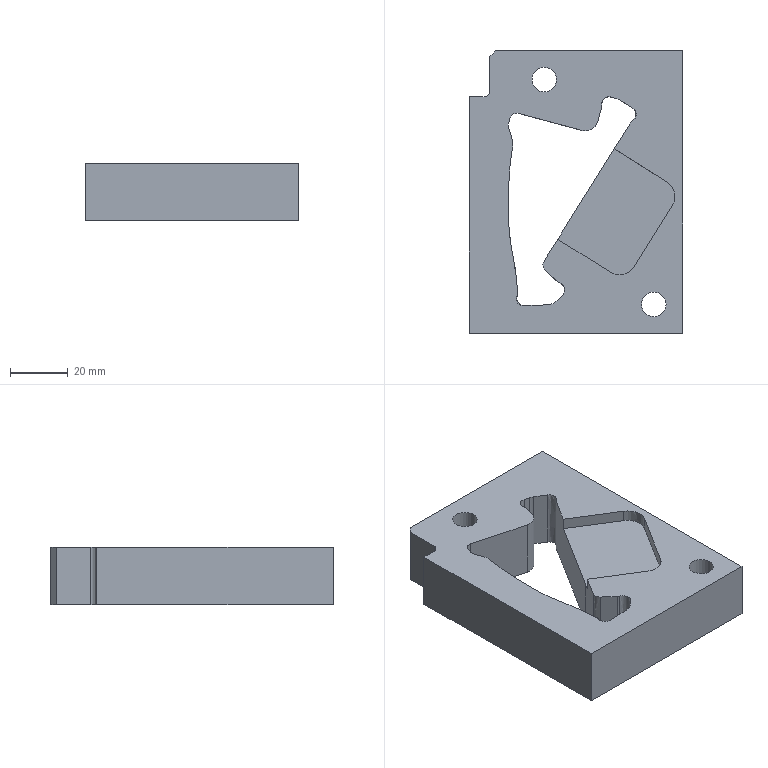Part | NX | features solid 2 | 1 solid | 52 faces | box 74 x 98 x 20 mm | volume 102751 mm3 | spline 21 | plane 18 | cylinder 13 | commonest cylinder face diameters 5 x2 8.5 x2 9 x2 11 x2 14 x2 4 x1